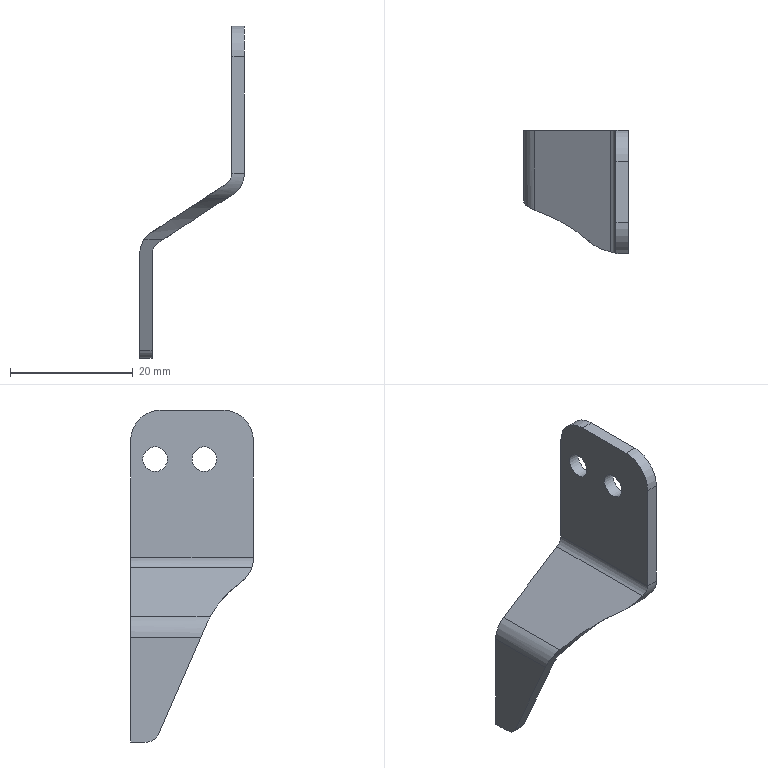Part | STEP file | 1-50 | 1 solid | 22 faces | box 17 x 20 x 54 mm | volume 1793 mm3 | plane 11 | cylinder 11 | commonest cylinder face diameters 4 x5 10 x3 8 x2 32 x1